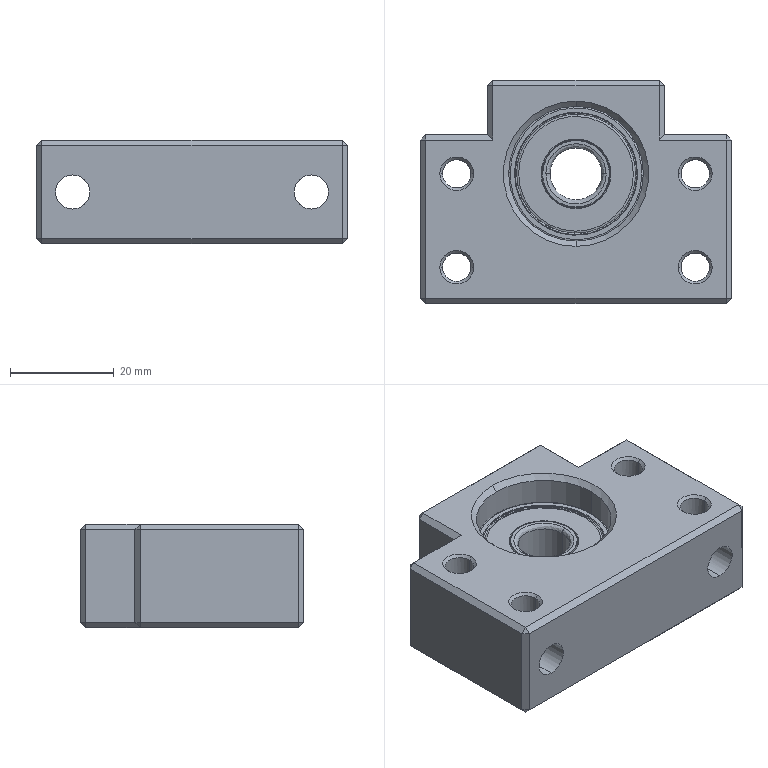Part | STEP file | Screw support seat BF12 | 13 solids | 218 faces | box 60 x 43 x 20 mm | volume 33949 mm3 | spline 78 | plane 58 | cylinder 54 | cone 28 | commonest cylinder face diameters 5.5 x16 23.5 x8 6.6 x4 10.8 x4 13.05 x4 13.47 x4